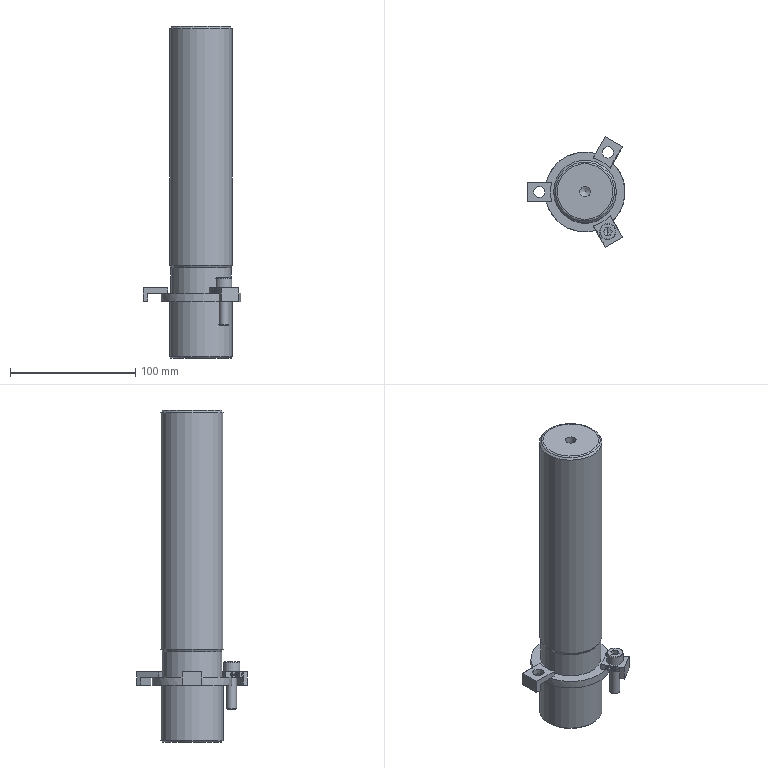Part | STEP file | lll_id3350_x_t | 1 solid | 196 faces | box 78.2 x 88.144 x 265 mm | volume 526178 mm3 | plane 118 | other 57 | cylinder 11 | cone 9 | torus 1 | commonest cylinder face diameters 9 x3 50 x2 8 x1 8.5 x1 10.5 x1 13 x1